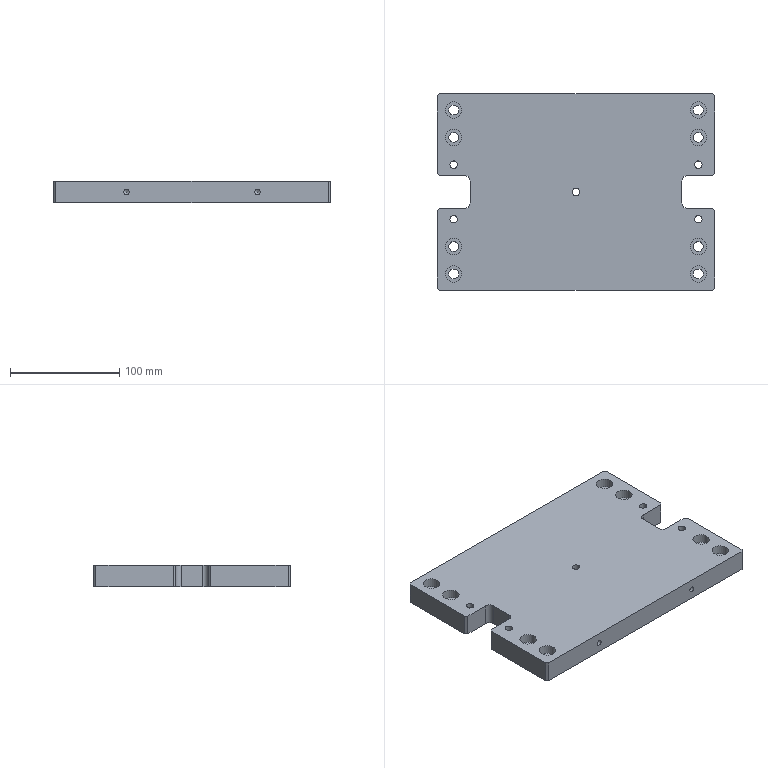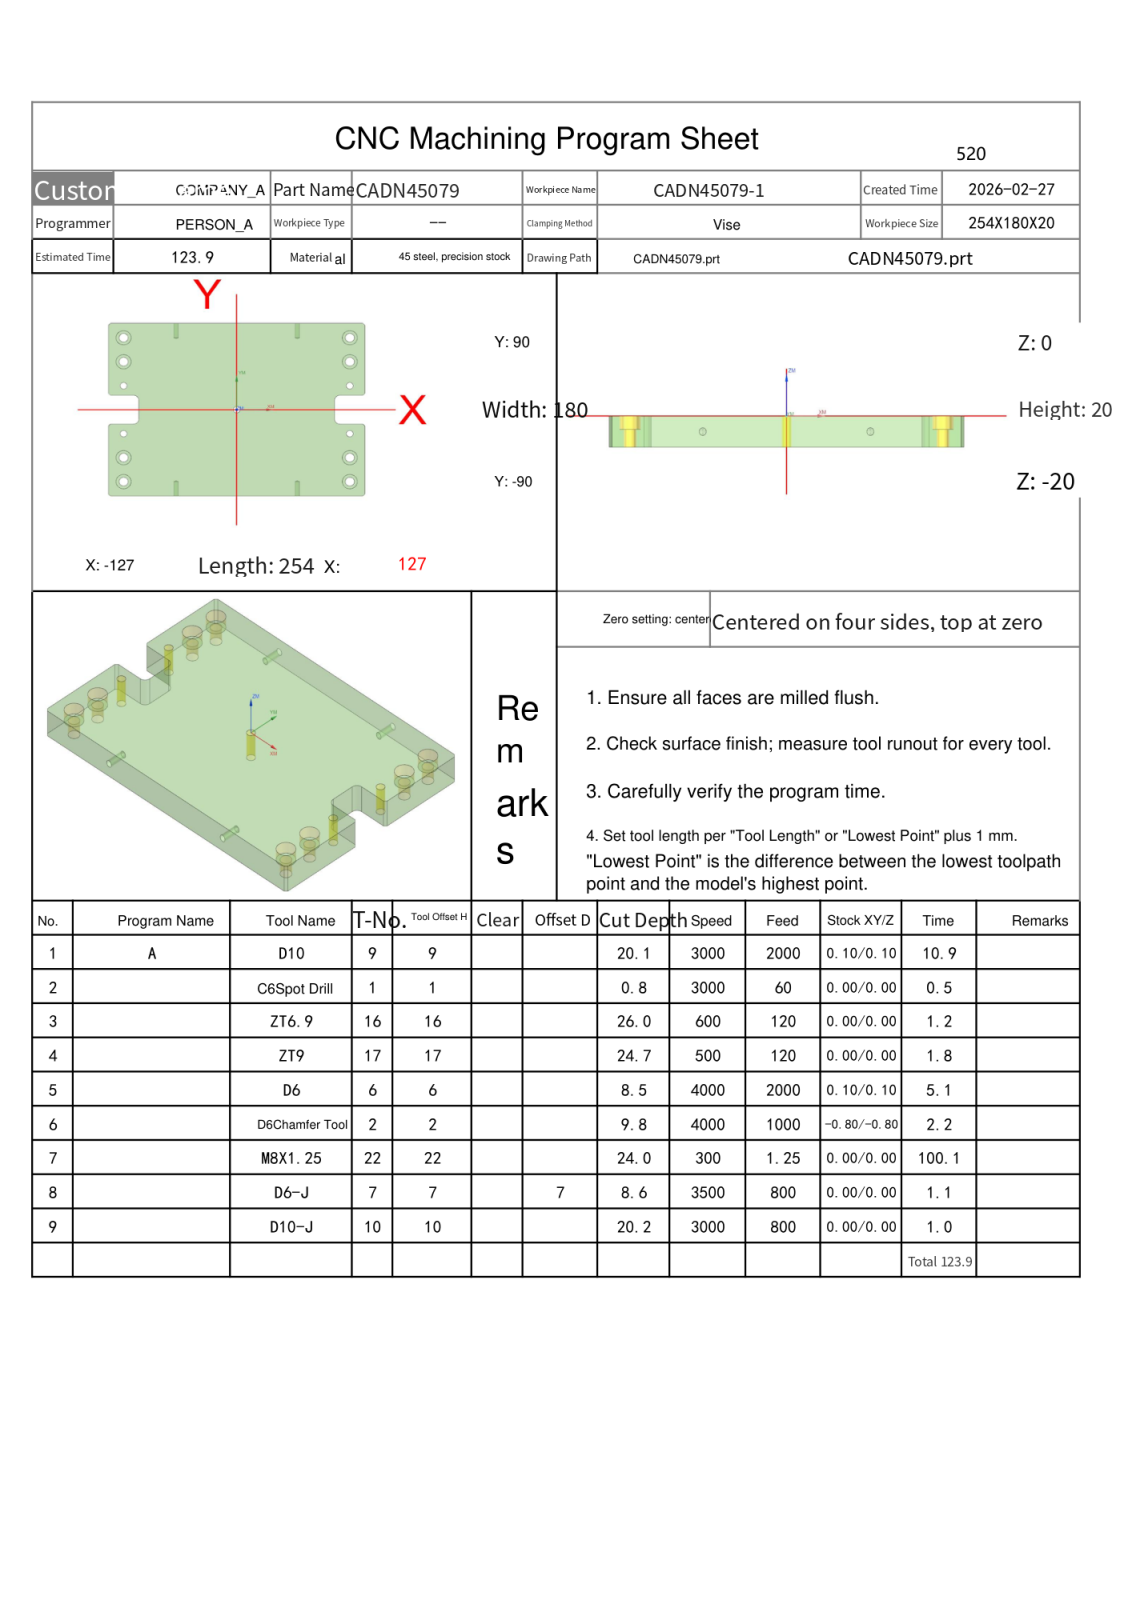NC program | NX | posted by the shop | part box 254 x 180 x 20 mm
Lines 4155 to 5116 of 5116:
N6 T02 M06
(D6Chamfer Tool  D=6. R=0. H=02 ce=-0.80 di=0.00)
G00 G90 G54 X-112.8 Y-23.5 M03 S4000
G43 H02 Z30.
M08
Z-1.
G01 Z-1.5 F500.
X-113.2
G03 X-114.7 Y-25. I0.0 J-1.5
X-112. Y-27.7 I2.7 J0.0
X-109.3 Y-25. I0.0 J2.7
X-112. Y-22.3 I-2.7 J0.0
X-114.7 Y-25. I0.0 J-2.7
X-113.2 Y-26.5 I1.5 J0.0
G01 X-112.8
Z-1.
G00 Z30.
Y26.5
Z-1.
G01 Z-1.5
X-113.2
G03 X-114.7 Y25. I0.0 J-1.5
X-112. Y22.3 I2.7 J0.0
X-109.3 Y25. I0.0 J2.7
X-112. Y27.7 I-2.7 J0.0
X-114.7 Y25. I0.0 J-2.7
X-113.2 Y23.5 I1.5 J0.0
G01 X-112.8
Z-1.
G00 Z30.
X-.8 Y1.5
Z-1.
G01 Z-1.5
X-1.2
G03 X-2.7 Y0.0 I0.0 J-1.5
X0.0 Y-2.7 I2.7 J0.0
X2.7 Y0.0 I0.0 J2.7
X0.0 Y2.7 I-2.7 J0.0
X-2.7 Y0.0 I0.0 J-2.7
X-1.2 Y-1.5 I1.5 J0.0
G01 X-.8
Z-1.
G00 Z30.
X111.2 Y26.5
Z-1.
G01 Z-1.5
X110.8
G03 X109.3 Y25. I0.0 J-1.5
X112. Y22.3 I2.7 J0.0
X114.7 Y25. I0.0 J2.7
X112. Y27.7 I-2.7 J0.0
X109.3 Y25. I0.0 J-2.7
X110.8 Y23.5 I1.5 J0.0
G01 X111.2
Z-1.
G00 Z30.
Y-23.5
Z-1.
G01 Z-1.5
X110.8
G03 X109.3 Y-25. I0.0 J-1.5
X112. Y-27.7 I2.7 J0.0
X114.7 Y-25. I0.0 J2.7
X112. Y-22.3 I-2.7 J0.0
X109.3 Y-25. I0.0 J-2.7
X110.8 Y-26.5 I1.5 J0.0
G01 X111.2
Z-1.
G00 Z30.
G00 G90 X.386 Y-91.227 M03 S3500
Z30.
Z.172
G01 Z-1.2 F1000.
G03 X.1 Y-91.027 I-1.286 J-1.532
G01 X.054 Y-90.997
X0.0 Y-91.
X-125.
X-125.259 Y-90.966
X-125.5 Y-90.866
X-125.707 Y-90.707
X-127.707 Y-88.707
X-127.866 Y-88.5
X-127.966 Y-88.259
X-128. Y-88.
Y-17.
X-127.966 Y-16.741
X-127.866 Y-16.5
X-127.707 Y-16.293
X-125.707 Y-14.293
X-125.5 Y-14.134
X-125.259 Y-14.034
X-125. Y-14.
X-102.
G03 X-98. Y-10. I0.0 J4.
G01 Y10.
G03 X-102. Y14. I-4. J0.0
G01 X-125.
X-125.259 Y14.034
X-125.5 Y14.134
X-125.707 Y14.293
X-127.707 Y16.293
X-127.866 Y16.5
X-127.966 Y16.741
X-128. Y17.
Y88.
X-127.966 Y88.259
X-127.866 Y88.5
X-127.707 Y88.707
X-125.707 Y90.707
X-125.5 Y90.866
X-125.259 Y90.966
X-125. Y91.
X125.
X125.259 Y90.966
X125.5 Y90.866
X125.707 Y90.707
X127.707 Y88.707
X127.866 Y88.5
X127.966 Y88.259
X128. Y88.
Y17.
X127.966 Y16.741
X127.866 Y16.5
X127.707 Y16.293
X125.707 Y14.293
X125.5 Y14.134
X125.259 Y14.034
X125. Y14.
X102.
G03 X98. Y10. I0.0 J-4.
G01 Y-10.
G03 X102. Y-14. I4. J0.0
G01 X125.
X125.259 Y-14.034
X125.5 Y-14.134
X125.707 Y-14.293
X127.707 Y-16.293
X127.866 Y-16.5
X127.966 Y-16.741
X128. Y-17.
Y-88.
X127.966 Y-88.259
X127.866 Y-88.5
X127.707 Y-88.707
X125.707 Y-90.707
X125.5 Y-90.866
X125.259 Y-90.966
X125. Y-91.
X0.0
X-.054 Y-90.997
X-.1 Y-91.027
G03 X-.386 Y-91.227 I1. J-1.732
G01 Z.172
G00 Z10.
X105.706 Y-74.603
Z.21
G01 Z-1.2
G03 X105.522 Y-74.899 I1.597 J-1.204
G01 X105.494 Y-74.946
X105.5 Y-75.
G03 X112. Y-81.5 I6.5 J0.0
X118.5 Y-75. I0.0 J6.5
X112. Y-68.5 I-6.5 J0.0
X105.5 Y-75. I0.0 J-6.5
G01 X105.494 Y-75.054
X105.522 Y-75.101
G03 X105.706 Y-75.397 I1.782 J.908
G01 Z.21
G00 Z10.
Y-49.603
Z.21
G01 Z-1.2
G03 X105.522 Y-49.899 I1.597 J-1.204
G01 X105.494 Y-49.946
X105.5 Y-50.
G03 X112. Y-56.5 I6.5 J0.0
X118.5 Y-50. I0.0 J6.5
X112. Y-43.5 I-6.5 J0.0
X105.5 Y-50. I0.0 J-6.5
G01 X105.494 Y-50.054
X105.522 Y-50.101
G03 X105.706 Y-50.397 I1.782 J.908
G01 Z.21
G00 Z10.
X109.792 Y-24.596
Z.252
G01 Z-1.2
G03 X109.618 Y-24.898 I1.638 J-1.147
G01 X109.592 Y-24.946
X109.6 Y-25.
G03 X112. Y-27.4 I2.4 J0.0
X114.4 Y-25. I0.0 J2.4
X112. Y-22.6 I-2.4 J0.0
X109.6 Y-25. I0.0 J-2.4
G01 X109.592 Y-25.054
X109.618 Y-25.102
G03 X109.792 Y-25.404 I1.813 J.845
G01 Z.252
G00 Z10.
Y25.404
Z.252
G01 Z-1.2
G03 X109.618 Y25.102 I1.638 J-1.147
G01 X109.592 Y25.054
X109.6 Y25.
G03 X112. Y22.6 I2.4 J0.0
X114.4 Y25. I0.0 J2.4
X112. Y27.4 I-2.4 J0.0
X109.6 Y25. I0.0 J-2.4
G01 X109.592 Y24.946
X109.618 Y24.898
G03 X109.792 Y24.596 I1.813 J.845
G01 Z.252
G00 Z10.
X105.706 Y50.397
Z.21
G01 Z-1.2
G03 X105.522 Y50.101 I1.597 J-1.204
G01 X105.494 Y50.054
X105.5 Y50.
G03 X112. Y43.5 I6.5 J0.0
X118.5 Y50. I0.0 J6.5
X112. Y56.5 I-6.5 J0.0
X105.5 Y50. I0.0 J-6.5
G01 X105.494 Y49.946
X105.522 Y49.899
G03 X105.706 Y49.603 I1.782 J.908
G01 Z.21
G00 Z10.
Y75.397
Z.21
G01 Z-1.2
G03 X105.522 Y75.101 I1.597 J-1.204
G01 X105.494 Y75.054
X105.5 Y75.
G03 X112. Y68.5 I6.5 J0.0
X118.5 Y75. I0.0 J6.5
X112. Y81.5 I-6.5 J0.0
X105.5 Y75. I0.0 J-6.5
G01 X105.494 Y74.946
X105.522 Y74.899
G03 X105.706 Y74.603 I1.782 J.908
G01 Z.21
G00 Z10.
X-2.208 Y.404
Z.252
G01 Z-1.2
G03 X-2.382 Y.102 I1.638 J-1.147
G01 X-2.408 Y.054
X-2.4 Y0.0
G03 X0.0 Y-2.4 I2.4 J0.0
X2.4 Y0.0 I0.0 J2.4
X0.0 Y2.4 I-2.4 J0.0
X-2.4 Y0.0 I0.0 J-2.4
G01 X-2.408 Y-.054
X-2.382 Y-.102
G03 X-2.208 Y-.404 I1.813 J.845
G01 Z.252
G00 Z10.
X-118.294 Y75.397
Z.21
G01 Z-1.2
G03 X-118.478 Y75.101 I1.597 J-1.204
G01 X-118.506 Y75.054
X-118.5 Y75.
G03 X-112. Y68.5 I6.5 J0.0
X-105.5 Y75. I0.0 J6.5
X-112. Y81.5 I-6.5 J0.0
X-118.5 Y75. I0.0 J-6.5
G01 X-118.506 Y74.946
X-118.478 Y74.899
G03 X-118.294 Y74.603 I1.782 J.908
G01 Z.21
G00 Z10.
Y50.397
Z.21
G01 Z-1.2
G03 X-118.478 Y50.101 I1.597 J-1.204
G01 X-118.506 Y50.054
X-118.5 Y50.
G03 X-112. Y43.5 I6.5 J0.0
X-105.5 Y50. I0.0 J6.5
X-112. Y56.5 I-6.5 J0.0
X-118.5 Y50. I0.0 J-6.5
G01 X-118.506 Y49.946
X-118.478 Y49.899
G03 X-118.294 Y49.603 I1.782 J.908
G01 Z.21
G00 Z10.
X-114.208 Y25.404
Z.252
G01 Z-1.2
G03 X-114.382 Y25.102 I1.638 J-1.147
G01 X-114.408 Y25.054
X-114.4 Y25.
G03 X-112. Y22.6 I2.4 J0.0
X-109.6 Y25. I0.0 J2.4
X-112. Y27.4 I-2.4 J0.0
X-114.4 Y25. I0.0 J-2.4
G01 X-114.408 Y24.946
X-114.382 Y24.898
G03 X-114.208 Y24.596 I1.813 J.845
G01 Z.252
G00 Z10.
Y-24.596
Z.252
G01 Z-1.2
G03 X-114.382 Y-24.898 I1.638 J-1.147
G01 X-114.408 Y-24.946
X-114.4 Y-25.
G03 X-112. Y-27.4 I2.4 J0.0
X-109.6 Y-25. I0.0 J2.4
X-112. Y-22.6 I-2.4 J0.0
X-114.4 Y-25. I0.0 J-2.4
G01 X-114.408 Y-25.054
X-114.382 Y-25.102
G03 X-114.208 Y-25.404 I1.813 J.845
G01 Z.252
G00 Z10.
X-118.294 Y-49.603
Z.21
G01 Z-1.2
G03 X-118.478 Y-49.899 I1.597 J-1.204
G01 X-118.506 Y-49.946
X-118.5 Y-50.
G03 X-112. Y-56.5 I6.5 J0.0
X-105.5 Y-50. I0.0 J6.5
X-112. Y-43.5 I-6.5 J0.0
X-118.5 Y-50. I0.0 J-6.5
G01 X-118.506 Y-50.054
X-118.478 Y-50.101
G03 X-118.294 Y-50.397 I1.782 J.908
G01 Z.21
G00 Z10.
Y-74.603
Z.21
G01 Z-1.2
G03 X-118.478 Y-74.899 I1.597 J-1.204
G01 X-118.506 Y-74.946
X-118.5 Y-75.
G03 X-112. Y-81.5 I6.5 J0.0
X-105.5 Y-75. I0.0 J6.5
X-112. Y-68.5 I-6.5 J0.0
X-118.5 Y-75. I0.0 J-6.5
G01 X-118.506 Y-75.054
X-118.478 Y-75.101
G03 X-118.294 Y-75.397 I1.782 J.908
G01 Z.21
G00 Z2.55
X-115.303 Y-74.599
Z-2.127
G01 Z-9.8
G03 X-115.481 Y-74.898 I1.624 J-1.167
G01 X-115.507 Y-74.946
X-115.5 Y-75.
G03 X-112. Y-78.5 I3.5 J0.0
X-108.5 Y-75. I0.0 J3.5
X-112. Y-71.5 I-3.5 J0.0
X-115.5 Y-75. I0.0 J-3.5
G01 X-115.507 Y-75.054
X-115.481 Y-75.102
G03 X-115.303 Y-75.401 I1.802 J.868
G01 Z-2.127
G00 Z10.
Y-49.599
Z-2.127
G01 Z-9.8
G03 X-115.481 Y-49.898 I1.624 J-1.167
G01 X-115.507 Y-49.946
X-115.5 Y-50.
G03 X-112. Y-53.5 I3.5 J0.0
X-108.5 Y-50. I0.0 J3.5
X-112. Y-46.5 I-3.5 J0.0
X-115.5 Y-50. I0.0 J-3.5
G01 X-115.507 Y-50.054
X-115.481 Y-50.102
G03 X-115.303 Y-50.401 I1.802 J.868
G01 Z-2.127
G00 Z10.
Y50.401
Z-2.127
G01 Z-9.8
G03 X-115.481 Y50.102 I1.624 J-1.167
G01 X-115.507 Y50.054
X-115.5 Y50.
G03 X-112. Y46.5 I3.5 J0.0
X-108.5 Y50. I0.0 J3.5
X-112. Y53.5 I-3.5 J0.0
X-115.5 Y50. I0.0 J-3.5
G01 X-115.507 Y49.946
X-115.481 Y49.898
G03 X-115.303 Y49.599 I1.802 J.868
G01 Z-2.127
G00 Z10.
Y75.401
Z-2.127
G01 Z-9.8
G03 X-115.481 Y75.102 I1.624 J-1.167
G01 X-115.507 Y75.054
X-115.5 Y75.
G03 X-112. Y71.5 I3.5 J0.0
X-108.5 Y75. I0.0 J3.5
X-112. Y78.5 I-3.5 J0.0
X-115.5 Y75. I0.0 J-3.5
G01 X-115.507 Y74.946
X-115.481 Y74.898
G03 X-115.303 Y74.599 I1.802 J.868
G01 Z-2.127
G00 Z10.
X108.697 Y75.401
Z-2.127
G01 Z-9.8
G03 X108.519 Y75.102 I1.624 J-1.167
G01 X108.493 Y75.054
X108.5 Y75.
G03 X112. Y71.5 I3.5 J0.0
X115.5 Y75. I0.0 J3.5
X112. Y78.5 I-3.5 J0.0
X108.5 Y75. I0.0 J-3.5
G01 X108.493 Y74.946
X108.519 Y74.898
G03 X108.697 Y74.599 I1.802 J.868
G01 Z-2.127
G00 Z10.
Y50.401
Z-2.127
G01 Z-9.8
G03 X108.519 Y50.102 I1.624 J-1.167
G01 X108.493 Y50.054
X108.5 Y50.
G03 X112. Y46.5 I3.5 J0.0
X115.5 Y50. I0.0 J3.5
X112. Y53.5 I-3.5 J0.0
X108.5 Y50. I0.0 J-3.5
G01 X108.493 Y49.946
X108.519 Y49.898
G03 X108.697 Y49.599 I1.802 J.868
G01 Z-2.127
G00 Z10.
Y-49.599
Z-2.127
G01 Z-9.8
G03 X108.519 Y-49.898 I1.624 J-1.167
G01 X108.493 Y-49.946
X108.5 Y-50.
G03 X112. Y-53.5 I3.5 J0.0
X115.5 Y-50. I0.0 J3.5
X112. Y-46.5 I-3.5 J0.0
X108.5 Y-50. I0.0 J-3.5
G01 X108.493 Y-50.054
X108.519 Y-50.102
G03 X108.697 Y-50.401 I1.802 J.868
G01 Z-2.127
G00 Z10.
Y-74.599
Z-2.127
G01 Z-9.8
G03 X108.519 Y-74.898 I1.624 J-1.167
G01 X108.493 Y-74.946
X108.5 Y-75.
G03 X112. Y-78.5 I3.5 J0.0
X115.5 Y-75. I0.0 J3.5
X112. Y-71.5 I-3.5 J0.0
X108.5 Y-75. I0.0 J-3.5
G01 X108.493 Y-75.054
X108.519 Y-75.102
G03 X108.697 Y-75.401 I1.802 J.868
G01 Z-2.127
G00 Z30.
G91 G28 Z0.0
M05
M09
G91 G28 Z0.0
M01
N7 T22 M06
(M8X1.25 D=6.8 DR_a=180 H=22)
G00 G90 G54 X-112. Y-25. M03 S300
G43 H22 Z30.
M08
G95
G98 G84 X-112. Y-25. Z-24. R1. F1.25 Q3.
Y25.
X0.0 Y0.0
X112. Y-25.
Y25.
G80
G94
G00 Z30.
G91 G28 Z0.0
M05
M09
G91 G28 Z0.0
M01
N8 T07 M06
(D6-J  D=6. R=0. H=07 ce=0.00 di=0.00)
G00 G90 G54 X109.58 Y46.25 M03 S3500
G43 H07 Z30.
M08
Z.5
G01 X109.704 Y46.165 Z.492 F800.
X110.192 Y45.912 Z.463
X110.708 Y45.721 Z.435
X111.242 Y45.595 Z.406
X111.789 Y45.535 Z.377
X112.211 Z.355
X112.804 Y45.603 Z.324
X113.382 Y45.749 Z.292
X113.935 Y45.971 Z.261
X114.454 Y46.264 Z.23
X114.929 Y46.624 Z.199
X115.353 Y47.044 Z.167
X115.716 Y47.516 Z.136
X116.014 Y48.033 Z.105
X116.24 Y48.585 Z.074
X116.39 Y49.162 Z.042
X116.463 Y49.753 Z.011
X116.465 Y49.965 Z0.0
G41 D07
X116.5 Y50.
G03 X112. Y54.5 Z-1.075 I-4.5 J0.0
X107.5 Y50. Z-2.15 I0.0 J-4.5
X112. Y45.5 Z-3.225 I4.5 J0.0
X116.5 Y50. Z-4.3 I0.0 J4.5
X112. Y54.5 Z-5.375 I-4.5 J0.0
X107.5 Y50. Z-6.45 I0.0 J-4.5
X112. Y45.5 Z-7.525 I4.5 J0.0
X116.5 Y50. Z-8.6 I0.0 J4.5
X112. Y54.5 I-4.5 J0.0
X107.5 Y50. I0.0 J-4.5
X112. Y45.5 I4.5 J0.0
X116.5 Y50. I0.0 J4.5
X116.482 Y50.399 I-4.5 J0.0
G01 X116.477 Y50.427
X116.456 Y50.445
X116.428
G40 X116.378 Y50.44
Z-7.6
G00 Z30.
X109.58 Y71.25
Z.5
G01 X109.704 Y71.165 Z.492
X110.192 Y70.912 Z.463
X110.708 Y70.721 Z.435
X111.242 Y70.595 Z.406
X111.789 Y70.535 Z.377
X112.211 Z.355
X112.804 Y70.603 Z.324
X113.382 Y70.749 Z.292
X113.935 Y70.971 Z.261
X114.454 Y71.264 Z.23
X114.929 Y71.624 Z.199
X115.353 Y72.044 Z.167
X115.716 Y72.516 Z.136
X116.014 Y73.033 Z.105
X116.24 Y73.585 Z.074
X116.39 Y74.162 Z.042
X116.463 Y74.753 Z.011
X116.465 Y74.965 Z0.0
G41 D07
X116.5 Y75.
G03 X112. Y79.5 Z-1.075 I-4.5 J0.0
X107.5 Y75. Z-2.15 I0.0 J-4.5
X112. Y70.5 Z-3.225 I4.5 J0.0
X116.5 Y75. Z-4.3 I0.0 J4.5
X112. Y79.5 Z-5.375 I-4.5 J0.0
X107.5 Y75. Z-6.45 I0.0 J-4.5
X112. Y70.5 Z-7.525 I4.5 J0.0
X116.5 Y75. Z-8.6 I0.0 J4.5
X112. Y79.5 I-4.5 J0.0
X107.5 Y75. I0.0 J-4.5
X112. Y70.5 I4.5 J0.0
X116.5 Y75. I0.0 J4.5
X116.482 Y75.399 I-4.5 J0.0
G01 X116.477 Y75.427
X116.456 Y75.445
X116.428
G40 X116.378 Y75.44
Z-7.6
G00 Z30.
X109.581 Y-78.751
Z.5
G01 X109.704 Y-78.835 Z.492
X110.192 Y-79.088 Z.463
X110.708 Y-79.279 Z.435
X111.242 Y-79.405 Z.406
X111.789 Y-79.465 Z.377
X112.211 Z.355
X112.793 Y-79.399 Z.324
X113.36 Y-79.258 Z.293
X113.904 Y-79.044 Z.263
X114.416 Y-78.76 Z.232
X114.886 Y-78.413 Z.202
X115.307 Y-78.007 Z.171
X115.672 Y-77.549 Z.14
X115.973 Y-77.048 Z.11
X116.149 Y-76.663 Z.087
X116.305 Y-76.203 Z.062
X116.41 Y-75.729 Z.037
X116.463 Y-75.247 Z.011
X116.465 Y-75.035 Z0.0
G41 D07
X116.5 Y-75.
G03 X112. Y-70.5 Z-1.075 I-4.5 J0.0
X107.5 Y-75. Z-2.15 I0.0 J-4.5
X112. Y-79.5 Z-3.225 I4.5 J0.0
X116.093 Y-76.87 Z-4.007 I0.0 J4.5
X116.5 Y-75. Z-4.3 I-4.093 J1.87
X112. Y-70.5 Z-5.375 I-4.5 J0.0
X107.5 Y-75. Z-6.45 I0.0 J-4.5
X112. Y-79.5 Z-7.525 I4.5 J0.0
X116.093 Y-76.87 Z-8.307 I0.0 J4.5
X116.5 Y-75. Z-8.6 I-4.093 J1.87
X112. Y-70.5 I-4.5 J0.0
X107.5 Y-75. I0.0 J-4.5
X112. Y-79.5 I4.5 J0.0
X116.5 Y-75. I0.0 J4.5
X116.482 Y-74.601 I-4.5 J0.0
G01 X116.477 Y-74.573
X116.456 Y-74.555
X116.428
G40 X116.378 Y-74.56
Z-7.6
G00 Z30.
X109.58 Y-53.75
Z.5
G01 X109.704 Y-53.835 Z.492
X110.192 Y-54.088 Z.463
X110.708 Y-54.279 Z.435
X111.242 Y-54.405 Z.406
X111.789 Y-54.465 Z.377
X112.211 Z.355
X112.804 Y-54.397 Z.324
X113.382 Y-54.251 Z.292
X113.935 Y-54.029 Z.261
X114.454 Y-53.736 Z.23
X114.929 Y-53.376 Z.199
X115.353 Y-52.956 Z.167
X115.716 Y-52.484 Z.136
X116.014 Y-51.967 Z.105
X116.24 Y-51.415 Z.074
X116.39 Y-50.838 Z.042
X116.463 Y-50.247 Z.011
X116.465 Y-50.035 Z0.0
G41 D07
X116.5 Y-50.
G03 X112. Y-45.5 Z-1.075 I-4.5 J0.0
X109.231 Y-46.453 Z-1.529 I0.0 J-4.5
X107.5 Y-50. Z-2.15 I2.769 J-3.547
X112. Y-54.5 Z-3.225 I4.5 J0.0
X116.5 Y-50. Z-4.3 I0.0 J4.5
X112. Y-45.5 Z-5.375 I-4.5 J0.0
X109.231 Y-46.453 Z-5.829 I0.0 J-4.5
X107.5 Y-50. Z-6.45 I2.769 J-3.547
X112. Y-54.5 Z-7.525 I4.5 J0.0
X116.5 Y-50. Z-8.6 I0.0 J4.5
X112. Y-45.5 I-4.5 J0.0
X107.5 Y-50. I0.0 J-4.5
X112. Y-54.5 I4.5 J0.0
X116.5 Y-50. I0.0 J4.5
X116.482 Y-49.601 I-4.5 J0.0
G01 X116.477 Y-49.573
X116.456 Y-49.555
X116.428
G40 X116.378 Y-49.56
Z-7.6
G00 Z30.
X-109.58 Y-46.25
Z.5
G01 X-109.704 Y-46.165 Z.492
X-110.192 Y-45.912 Z.463
X-110.708 Y-45.721 Z.435
X-111.242 Y-45.595 Z.406
X-111.789 Y-45.535 Z.377
X-112.211 Z.355
X-112.804 Y-45.603 Z.324
X-113.382 Y-45.749 Z.292
X-113.935 Y-45.971 Z.261
X-114.454 Y-46.264 Z.23
X-114.929 Y-46.624 Z.199
X-115.353 Y-47.044 Z.167
X-115.716 Y-47.516 Z.136
X-116.014 Y-48.033 Z.105
X-116.24 Y-48.585 Z.074
X-116.39 Y-49.162 Z.042
X-116.463 Y-49.753 Z.011
X-116.465 Y-49.965 Z0.0
G41 D07
X-116.5 Y-50.
G03 X-112. Y-54.5 Z-1.075 I4.5 J0.0
X-107.5 Y-50. Z-2.15 I0.0 J4.5
X-112. Y-45.5 Z-3.225 I-4.5 J0.0
X-116.5 Y-50. Z-4.3 I0.0 J-4.5
X-112. Y-54.5 Z-5.375 I4.5 J0.0
X-107.5 Y-50. Z-6.45 I0.0 J4.5
X-112. Y-45.5 Z-7.525 I-4.5 J0.0
X-116.5 Y-50. Z-8.6 I0.0 J-4.5
X-112. Y-54.5 I4.5 J0.0
X-107.5 Y-50. I0.0 J4.5
X-112. Y-45.5 I-4.5 J0.0
X-116.5 Y-50. I0.0 J-4.5
X-116.482 Y-50.399 I4.5 J0.0
G01 X-116.477 Y-50.427
X-116.456 Y-50.445
X-116.428
G40 X-116.378 Y-50.44
Z-7.6
G00 Z30.
X-109.58 Y-71.25
Z.5
G01 X-109.704 Y-71.165 Z.492
X-110.192 Y-70.912 Z.463
X-110.708 Y-70.721 Z.435
X-111.242 Y-70.595 Z.406
X-111.789 Y-70.535 Z.377
X-112.211 Z.355
X-112.804 Y-70.603 Z.324
X-113.382 Y-70.749 Z.292
X-113.935 Y-70.971 Z.261
X-114.454 Y-71.264 Z.23
X-114.929 Y-71.624 Z.199
X-115.353 Y-72.044 Z.167
X-115.716 Y-72.516 Z.136
X-116.014 Y-73.033 Z.105
X-116.24 Y-73.585 Z.074
X-116.39 Y-74.162 Z.042
X-116.463 Y-74.753 Z.011
X-116.465 Y-74.965 Z0.0
G41 D07
X-116.5 Y-75.
G03 X-112. Y-79.5 Z-1.075 I4.5 J0.0
X-107.5 Y-75. Z-2.15 I0.0 J4.5
X-112. Y-70.5 Z-3.225 I-4.5 J0.0
X-116.5 Y-75. Z-4.3 I0.0 J-4.5
X-112. Y-79.5 Z-5.375 I4.5 J0.0
X-107.5 Y-75. Z-6.45 I0.0 J4.5
X-112. Y-70.5 Z-7.525 I-4.5 J0.0
X-116.5 Y-75. Z-8.6 I0.0 J-4.5
X-112. Y-79.5 I4.5 J0.0
X-107.5 Y-75. I0.0 J4.5
X-112. Y-70.5 I-4.5 J0.0
X-116.5 Y-75. I0.0 J-4.5
X-116.482 Y-75.399 I4.5 J0.0
G01 X-116.477 Y-75.427
X-116.456 Y-75.445
X-116.428
G40 X-116.378 Y-75.44
Z-7.6
G00 Z30.
X-109.58 Y78.75
Z.5
G01 X-109.704 Y78.835 Z.492
X-110.192 Y79.088 Z.463
X-110.708 Y79.279 Z.435
X-111.242 Y79.405 Z.406
X-111.789 Y79.465 Z.377
X-112.211 Z.355
X-112.804 Y79.397 Z.324
X-113.382 Y79.251 Z.292
X-113.935 Y79.029 Z.261
X-114.454 Y78.736 Z.23
X-114.929 Y78.376 Z.199
X-115.353 Y77.956 Z.167
X-115.716 Y77.484 Z.136
X-116.014 Y76.967 Z.105
X-116.24 Y76.415 Z.074
X-116.39 Y75.838 Z.042
X-116.463 Y75.247 Z.011
X-116.465 Y75.035 Z0.0
G41 D07
X-116.5 Y75.
G03 X-112. Y70.5 Z-1.075 I4.5 J0.0
X-107.5 Y75. Z-2.15 I0.0 J4.5
X-112. Y79.5 Z-3.225 I-4.5 J0.0
X-116.5 Y75. Z-4.3 I0.0 J-4.5
X-112. Y70.5 Z-5.375 I4.5 J0.0
X-107.5 Y75. Z-6.45 I0.0 J4.5
X-112. Y79.5 Z-7.525 I-4.5 J0.0
X-116.5 Y75. Z-8.6 I0.0 J-4.5
X-112. Y70.5 I4.5 J0.0
X-107.5 Y75. I0.0 J4.5
X-112. Y79.5 I-4.5 J0.0
X-116.5 Y75. I0.0 J-4.5
X-116.482 Y74.601 I4.5 J0.0
G01 X-116.477 Y74.573
X-116.456 Y74.555
X-116.428
G40 X-116.378 Y74.56
Z-7.6
G00 Z30.
X-109.58 Y53.75
Z.5
G01 X-109.704 Y53.835 Z.492
X-110.192 Y54.088 Z.463
X-110.708 Y54.279 Z.435
X-111.242 Y54.405 Z.406
X-111.789 Y54.465 Z.377
X-112.211 Z.355
X-112.804 Y54.397 Z.324
X-113.382 Y54.251 Z.292
X-113.935 Y54.029 Z.261
X-114.454 Y53.736 Z.23
X-114.929 Y53.376 Z.199
X-115.353 Y52.956 Z.167
X-115.716 Y52.484 Z.136
X-116.014 Y51.967 Z.105
X-116.24 Y51.415 Z.074
X-116.39 Y50.838 Z.042
X-116.463 Y50.247 Z.011
X-116.465 Y50.035 Z0.0
G41 D07
X-116.5 Y50.
G03 X-112. Y45.5 Z-1.075 I4.5 J0.0
X-107.5 Y50. Z-2.15 I0.0 J4.5
X-112. Y54.5 Z-3.225 I-4.5 J0.0
X-116.5 Y50. Z-4.3 I0.0 J-4.5
X-112. Y45.5 Z-5.375 I4.5 J0.0
X-107.5 Y50. Z-6.45 I0.0 J4.5
X-112. Y54.5 Z-7.525 I-4.5 J0.0
X-116.5 Y50. Z-8.6 I0.0 J-4.5
X-112. Y45.5 I4.5 J0.0
X-107.5 Y50. I0.0 J4.5
X-112. Y54.5 I-4.5 J0.0
X-116.5 Y50. I0.0 J-4.5
X-116.482 Y49.601 I4.5 J0.0
G01 X-116.477 Y49.573
X-116.456 Y49.555
X-116.428
G40 X-116.378 Y49.56
Z-7.6
G00 Z30.
G91 G28 Z0.0
M05
M09
G91 G28 Z0.0
M01
N9 T10 M06
(D10-J  D=10. R=0. H=10 ce=0.00 di=0.00)
G00 G90 G54 X-124.293 Y-97.778 M03 S3000
G43 H10 Z30.
M08
Z-10.
G01 Z-11. F800.
X-128.536 Y-93.536
X-130.536 Y-91.536
X-134.778 Y-87.293
Z-10.
G00 Z30.
Y87.293
Z-10.
G01 Z-11.
X-130.536 Y91.536
X-128.536 Y93.536
X-124.293 Y97.778
Z-10.
G00 Z30.
X124.293
Z-10.
G01 Z-11.
X128.536 Y93.536
X130.536 Y91.536
X134.778 Y87.293
Z-10.
G00 Z30.
Y-87.293
Z-10.
G01 Z-11.
X130.536 Y-91.536
X128.536 Y-93.536
X124.293 Y-97.778
Z-10.
G00 Z30.
G00 G90 X-134.778 Y-17.707 M03 S3000
Z30.
Z-7.
G01 Z-8. F800.
X-130.536 Y-13.464
X-128.536 Y-11.464
G02 X-125. Y-10. I3.536 J-3.536
G01 X-102.
Y10.
X-125.
G02 X-128.536 Y11.464 I0.0 J5.
G01 X-130.536 Y13.464
X-134.778 Y17.707
Z-7.
G00 Z30.
Y-17.707
Z-15.
G01 Z-16.
X-130.536 Y-13.464
X-128.536 Y-11.464
G02 X-125. Y-10. I3.536 J-3.536
G01 X-102.
Y10.
X-125.
G02 X-128.536 Y11.464 I0.0 J5.
G01 X-130.536 Y13.464
X-134.778 Y17.707
Z-15.
G00 Z30.
Y-17.707
Z-19.2
G01 Z-20.2
X-130.536 Y-13.464
X-128.536 Y-11.464
G02 X-125. Y-10. I3.536 J-3.536
G01 X-102.
Y10.
X-125.
G02 X-128.536 Y11.464 I0.0 J5.
G01 X-130.536 Y13.464
X-134.778 Y17.707
Z-19.2
G00 Z30.
X134.778
Z-7.
G01 Z-8.
X130.536 Y13.464
X128.536 Y11.464
G02 X125. Y10. I-3.536 J3.536
G01 X102.
Y-10.
X125.
G02 X128.536 Y-11.464 I0.0 J-5.
G01 X130.536 Y-13.464
X134.778 Y-17.707
Z-7.
G00 Z30.
Y17.707
Z-15.
G01 Z-16.
X130.536 Y13.464
X128.536 Y11.464
G02 X125. Y10. I-3.536 J3.536
G01 X102.
Y-10.
X125.
G02 X128.536 Y-11.464 I0.0 J-5.
G01 X130.536 Y-13.464
X134.778 Y-17.707
Z-15.
G00 Z30.
Y17.707
Z-19.2
G01 Z-20.2
X130.536 Y13.464
X128.536 Y11.464
G02 X125. Y10. I-3.536 J3.536
G01 X102.
Y-10.
X125.
G02 X128.536 Y-11.464 I0.0 J-5.
G01 X130.536 Y-13.464
X134.778 Y-17.707
Z-19.2
G00 Z30.
M05
M09
G91 G28 Z0.0
G91 G28 Y0.0
M30
%